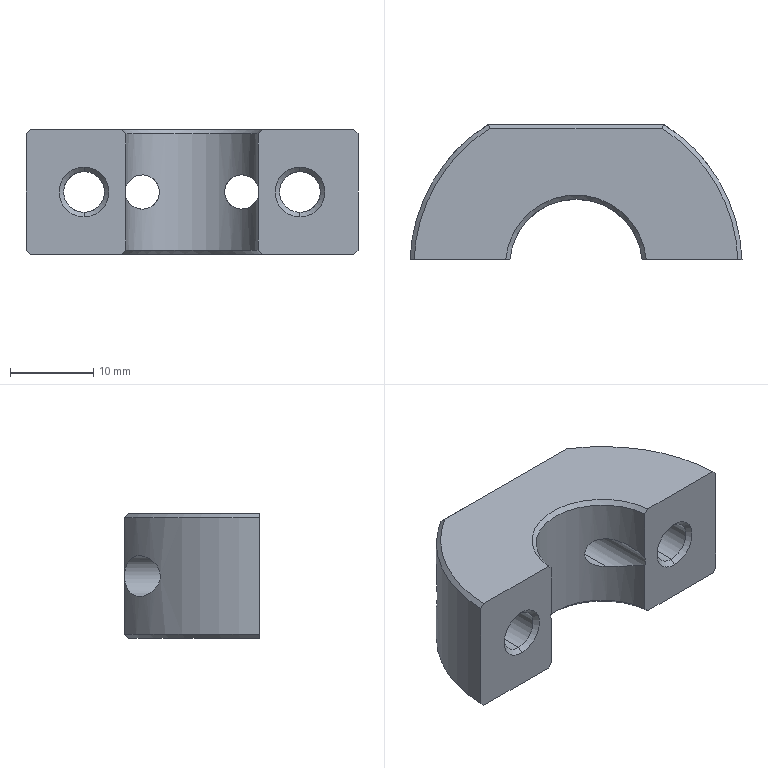Part | STEP file | 4 | 1 solid | 32 faces | box 39.972 x 16.25 x 15 mm | volume 6108 mm3 | cone 14 | cylinder 11 | plane 7 | commonest cylinder face diameters 4.134 x4 4.917 x4 40 x2 16 x1